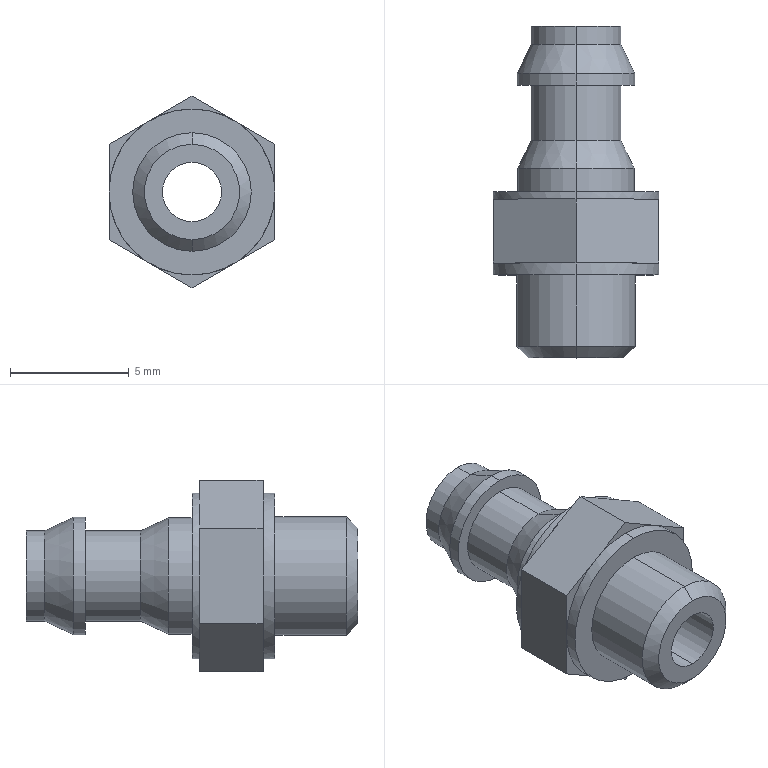Part | STEP file | M-5AU-6 | 1 solid | 45 faces | box 7 x 14 x 8.083 mm | volume 243.361 mm3 | plane 23 | cylinder 16 | cone 6 | commonest cylinder face diameters 3.8 x4 7 x4 2.5 x2 4.9 x2 4.95 x2 5 x2
STEP:
#1=CARTESIAN_POINT('',(0.,14.,1.25));
#2=VERTEX_POINT('',#1);
#3=CARTESIAN_POINT('',(0.,14.,-1.25));
#4=VERTEX_POINT('',#3);
#5=CARTESIAN_POINT('',(0.,14.,0.));
#6=DIRECTION('',(0.,-1.,0.));
#7=DIRECTION('',(0.,0.,-1.));
#8=AXIS2_PLACEMENT_3D('',#5,#6,#7);
#9=CIRCLE('',#8,1.25);
#10=EDGE_CURVE('',#2,#4,#9,.T.);
#11=ORIENTED_EDGE('',*,*,#10,.F.);
#12=CARTESIAN_POINT('',(0.,0.,1.25));
#13=VERTEX_POINT('',#12);
#14=CARTESIAN_POINT('',(0.,0.,1.25));
#15=DIRECTION('',(0.,-1.,0.));
#16=VECTOR('',#15,1000.);
#17=LINE('',#14,#16);
#18=EDGE_CURVE('',#2,#13,#17,.T.);
#19=ORIENTED_EDGE('',*,*,#18,.T.);
#20=CARTESIAN_POINT('',(0.,0.,-1.25));
#21=VERTEX_POINT('',#20);
#22=CARTESIAN_POINT('',(0.,0.,0.));
#23=DIRECTION('',(0.,1.,0.));
#24=DIRECTION('',(0.,0.,-1.));
#25=AXIS2_PLACEMENT_3D('',#22,#23,#24);
#26=CIRCLE('',#25,1.25);
#27=EDGE_CURVE('',#21,#13,#26,.T.);
#28=ORIENTED_EDGE('',*,*,#27,.F.);
#29=CARTESIAN_POINT('',(0.,0.,-1.25));
#30=DIRECTION('',(0.,-1.,0.));
#31=VECTOR('',#30,1000.);
#32=LINE('',#29,#31);
#33=EDGE_CURVE('',#4,#21,#32,.T.);
#34=ORIENTED_EDGE('',*,*,#33,.F.);
#35=EDGE_LOOP('',(#11,#19,#28,#34));
#36=FACE_OUTER_BOUND('',#35,.T.);
#37=CARTESIAN_POINT('',(0.,0.,0.));
#38=DIRECTION('',(0.,-1.,0.));
#39=DIRECTION('',(0.,0.,-1.));
#40=AXIS2_PLACEMENT_3D('',#37,#38,#39);
#41=CYLINDRICAL_SURFACE('',#40,1.25);
#42=ADVANCED_FACE('',(#36),#41,.F.);
#43=CARTESIAN_POINT('',(0.,14.,1.9));
#44=VERTEX_POINT('',#43);
#45=CARTESIAN_POINT('',(0.,14.,-1.9));
#46=VERTEX_POINT('',#45);
#47=CARTESIAN_POINT('',(0.,14.,0.));
#48=DIRECTION('',(0.,1.,0.));
#49=DIRECTION('',(0.,0.,-1.));
#50=AXIS2_PLACEMENT_3D('',#47,#48,#49);
#51=CIRCLE('',#50,1.9);
#52=EDGE_CURVE('',#44,#46,#51,.T.);
#53=ORIENTED_EDGE('',*,*,#52,.F.);
#54=CARTESIAN_POINT('',(0.,13.233,1.9));
#55=VERTEX_POINT('',#54);
#56=CARTESIAN_POINT('',(0.,13.617,1.9));
#57=DIRECTION('',(0.,-1.,0.));
#58=VECTOR('',#57,1000.);
#59=LINE('',#56,#58);
#60=EDGE_CURVE('',#44,#55,#59,.T.);
#61=ORIENTED_EDGE('',*,*,#60,.T.);
#62=CARTESIAN_POINT('',(0.,13.233,-1.9));
#63=VERTEX_POINT('',#62);
#64=CARTESIAN_POINT('',(0.,13.233,0.));
#65=DIRECTION('',(0.,1.,0.));
#66=DIRECTION('',(0.,0.,-1.));
#67=AXIS2_PLACEMENT_3D('',#64,#65,#66);
#68=CIRCLE('',#67,1.9);
#69=EDGE_CURVE('',#55,#63,#68,.T.);
#70=ORIENTED_EDGE('',*,*,#69,.T.);
#71=CARTESIAN_POINT('',(0.,13.617,-1.9));
#72=DIRECTION('',(0.,-1.,0.));
#73=VECTOR('',#72,1000.);
#74=LINE('',#71,#73);
#75=EDGE_CURVE('',#46,#63,#74,.T.);
#76=ORIENTED_EDGE('',*,*,#75,.F.);
#77=EDGE_LOOP('',(#53,#61,#70,#76));
#78=FACE_OUTER_BOUND('',#77,.T.);
#79=CARTESIAN_POINT('',(0.,13.617,0.));
#80=DIRECTION('',(0.,-1.,0.));
#81=DIRECTION('',(0.,0.,-1.));
#82=AXIS2_PLACEMENT_3D('',#79,#80,#81);
#83=CYLINDRICAL_SURFACE('',#82,1.9);
#84=ADVANCED_FACE('',(#78),#83,.T.);
#85=CARTESIAN_POINT('',(0.,0.,-2.01));
#86=VERTEX_POINT('',#85);
#87=CARTESIAN_POINT('',(0.,0.,2.01));
#88=VERTEX_POINT('',#87);
#89=CARTESIAN_POINT('',(0.,0.,0.));
#90=DIRECTION('',(0.,-1.,0.));
#91=DIRECTION('',(0.,0.,1.));
#92=AXIS2_PLACEMENT_3D('',#89,#90,#91);
#93=CIRCLE('',#92,2.01);
#94=EDGE_CURVE('',#86,#88,#93,.T.);
#95=ORIENTED_EDGE('',*,*,#94,.F.);
#96=CARTESIAN_POINT('',(0.,0.49,-2.5));
#97=VERTEX_POINT('',#96);
#98=CARTESIAN_POINT('',(0.,0.49,-2.5));
#99=DIRECTION('',(0.,0.7071,-0.7071));
#100=VECTOR('',#99,1000.);
#101=LINE('',#98,#100);
#102=EDGE_CURVE('',#86,#97,#101,.T.);
#103=ORIENTED_EDGE('',*,*,#102,.T.);
#104=CARTESIAN_POINT('',(0.,0.49,2.5));
#105=VERTEX_POINT('',#104);
#106=CARTESIAN_POINT('',(0.,0.49,0.));
#107=DIRECTION('',(0.,-1.,0.));
#108=DIRECTION('',(1.,0.,0.));
#109=AXIS2_PLACEMENT_3D('',#106,#107,#108);
#110=CIRCLE('',#109,2.5);
#111=EDGE_CURVE('',#97,#105,#110,.T.);
#112=ORIENTED_EDGE('',*,*,#111,.T.);
#113=CARTESIAN_POINT('',(0.,0.49,2.5));
#114=DIRECTION('',(0.,0.7071,0.7071));
#115=VECTOR('',#114,1000.);
#116=LINE('',#113,#115);
#117=EDGE_CURVE('',#88,#105,#116,.T.);
#118=ORIENTED_EDGE('',*,*,#117,.F.);
#119=EDGE_LOOP('',(#95,#103,#112,#118));
#120=FACE_OUTER_BOUND('',#119,.T.);
#121=CARTESIAN_POINT('',(0.,0.49,0.));
#122=DIRECTION('',(0.,1.,0.));
#123=DIRECTION('',(0.,0.,1.));
#124=AXIS2_PLACEMENT_3D('',#121,#122,#123);
#125=CONICAL_SURFACE('',#124,2.5,0.7854);
#126=ADVANCED_FACE('',(#120),#125,.T.);
#127=ORIENTED_EDGE('',*,*,#69,.F.);
#128=CARTESIAN_POINT('',(0.,12.,2.475));
#129=VERTEX_POINT('',#128);
#130=CARTESIAN_POINT('',(0.,12.,2.475));
#131=DIRECTION('',(0.,-0.9063,0.4226));
#132=VECTOR('',#131,1000.);
#133=LINE('',#130,#132);
#134=EDGE_CURVE('',#55,#129,#133,.T.);
#135=ORIENTED_EDGE('',*,*,#134,.T.);
#136=CARTESIAN_POINT('',(0.,12.,-2.475));
#137=VERTEX_POINT('',#136);
#138=CARTESIAN_POINT('',(0.,12.,0.));
#139=DIRECTION('',(0.,1.,0.));
#140=DIRECTION('',(1.,0.,0.));
#141=AXIS2_PLACEMENT_3D('',#138,#139,#140);
#142=CIRCLE('',#141,2.475);
#143=EDGE_CURVE('',#129,#137,#142,.T.);
#144=ORIENTED_EDGE('',*,*,#143,.T.);
#145=CARTESIAN_POINT('',(0.,12.,-2.475));
#146=DIRECTION('',(0.,-0.9063,-0.4226));
#147=VECTOR('',#146,1000.);
#148=LINE('',#145,#147);
#149=EDGE_CURVE('',#63,#137,#148,.T.);
#150=ORIENTED_EDGE('',*,*,#149,.F.);
#151=EDGE_LOOP('',(#127,#135,#144,#150));
#152=FACE_OUTER_BOUND('',#151,.T.);
#153=CARTESIAN_POINT('',(0.,12.,0.));
#154=DIRECTION('',(0.,-1.,0.));
#155=DIRECTION('',(0.,0.,-1.));
#156=AXIS2_PLACEMENT_3D('',#153,#154,#155);
#157=CONICAL_SURFACE('',#156,2.475,0.4363);
#158=ADVANCED_FACE('',(#152),#157,.T.);
#159=CARTESIAN_POINT('',(0.,3.5,-2.5));
#160=VERTEX_POINT('',#159);
#161=CARTESIAN_POINT('',(0.,3.5,2.5));
#162=VERTEX_POINT('',#161);
#163=CARTESIAN_POINT('',(0.,3.5,0.));
#164=DIRECTION('',(0.,-1.,0.));
#165=DIRECTION('',(0.,0.,-1.));
#166=AXIS2_PLACEMENT_3D('',#163,#164,#165);
#167=CIRCLE('',#166,2.5);
#168=EDGE_CURVE('',#160,#162,#167,.T.);
#169=ORIENTED_EDGE('',*,*,#168,.T.);
#170=CARTESIAN_POINT('',(0.,1.995,2.5));
#171=DIRECTION('',(0.,-1.,0.));
#172=VECTOR('',#171,1000.);
#173=LINE('',#170,#172);
#174=EDGE_CURVE('',#162,#105,#173,.T.);
#175=ORIENTED_EDGE('',*,*,#174,.T.);
#176=ORIENTED_EDGE('',*,*,#111,.F.);
#177=CARTESIAN_POINT('',(0.,1.995,-2.5));
#178=DIRECTION('',(0.,-1.,0.));
#179=VECTOR('',#178,1000.);
#180=LINE('',#177,#179);
#181=EDGE_CURVE('',#160,#97,#180,.T.);
#182=ORIENTED_EDGE('',*,*,#181,.F.);
#183=EDGE_LOOP('',(#169,#175,#176,#182));
#184=FACE_OUTER_BOUND('',#183,.T.);
#185=CARTESIAN_POINT('',(0.,1.995,0.));
#186=DIRECTION('',(0.,-1.,0.));
#187=DIRECTION('',(0.,0.,-1.));
#188=AXIS2_PLACEMENT_3D('',#185,#186,#187);
#189=CYLINDRICAL_SURFACE('',#188,2.5);
#190=ADVANCED_FACE('',(#184),#189,.T.);
#191=ORIENTED_EDGE('',*,*,#143,.F.);
#192=CARTESIAN_POINT('',(0.,11.5,2.475));
#193=VERTEX_POINT('',#192);
#194=CARTESIAN_POINT('',(0.,11.75,2.475));
#195=DIRECTION('',(0.,-1.,0.));
#196=VECTOR('',#195,1000.);
#197=LINE('',#194,#196);
#198=EDGE_CURVE('',#129,#193,#197,.T.);
#199=ORIENTED_EDGE('',*,*,#198,.T.);
#200=CARTESIAN_POINT('',(0.,11.5,-2.475));
#201=VERTEX_POINT('',#200);
#202=CARTESIAN_POINT('',(0.,11.5,0.));
#203=DIRECTION('',(0.,1.,0.));
#204=DIRECTION('',(0.,0.,-1.));
#205=AXIS2_PLACEMENT_3D('',#202,#203,#204);
#206=CIRCLE('',#205,2.475);
#207=EDGE_CURVE('',#193,#201,#206,.T.);
#208=ORIENTED_EDGE('',*,*,#207,.T.);
#209=CARTESIAN_POINT('',(0.,11.75,-2.475));
#210=DIRECTION('',(0.,-1.,0.));
#211=VECTOR('',#210,1000.);
#212=LINE('',#209,#211);
#213=EDGE_CURVE('',#137,#201,#212,.T.);
#214=ORIENTED_EDGE('',*,*,#213,.F.);
#215=EDGE_LOOP('',(#191,#199,#208,#214));
#216=FACE_OUTER_BOUND('',#215,.T.);
#217=CARTESIAN_POINT('',(0.,11.75,0.));
#218=DIRECTION('',(0.,-1.,0.));
#219=DIRECTION('',(0.,0.,-1.));
#220=AXIS2_PLACEMENT_3D('',#217,#218,#219);
#221=CYLINDRICAL_SURFACE('',#220,2.475);
#222=ADVANCED_FACE('',(#216),#221,.T.);
#223=CARTESIAN_POINT('',(1.75,4.,3.031));
#224=VERTEX_POINT('',#223);
#225=CARTESIAN_POINT('',(0.,4.,3.5));
#226=VERTEX_POINT('',#225);
#227=CARTESIAN_POINT('',(0.,4.,0.));
#228=DIRECTION('',(0.,-1.,0.));
#229=DIRECTION('',(0.,0.,-1.));
#230=AXIS2_PLACEMENT_3D('',#227,#228,#229);
#231=CIRCLE('',#230,3.5);
#232=EDGE_CURVE('',#224,#226,#231,.T.);
#233=ORIENTED_EDGE('',*,*,#232,.T.);
#234=CARTESIAN_POINT('',(0.,3.5,3.5));
#235=VERTEX_POINT('',#234);
#236=CARTESIAN_POINT('',(0.,3.75,3.5));
#237=DIRECTION('',(0.,-1.,0.));
#238=VECTOR('',#237,1000.);
#239=LINE('',#236,#238);
#240=EDGE_CURVE('',#226,#235,#239,.T.);
#241=ORIENTED_EDGE('',*,*,#240,.T.);
#242=CARTESIAN_POINT('',(0.,3.5,-3.5));
#243=VERTEX_POINT('',#242);
#244=CARTESIAN_POINT('',(0.,3.5,0.));
#245=DIRECTION('',(0.,-1.,0.));
#246=DIRECTION('',(0.,0.,-1.));
#247=AXIS2_PLACEMENT_3D('',#244,#245,#246);
#248=CIRCLE('',#247,3.5);
#249=EDGE_CURVE('',#243,#235,#248,.T.);
#250=ORIENTED_EDGE('',*,*,#249,.F.);
#251=CARTESIAN_POINT('',(0.,4.,-3.5));
#252=VERTEX_POINT('',#251);
#253=CARTESIAN_POINT('',(0.,3.75,-3.5));
#254=DIRECTION('',(0.,-1.,0.));
#255=VECTOR('',#254,1000.);
#256=LINE('',#253,#255);
#257=EDGE_CURVE('',#252,#243,#256,.T.);
#258=ORIENTED_EDGE('',*,*,#257,.F.);
#259=CARTESIAN_POINT('',(1.75,4.,-3.031));
#260=VERTEX_POINT('',#259);
#261=CARTESIAN_POINT('',(0.,4.,0.));
#262=DIRECTION('',(0.,-1.,0.));
#263=DIRECTION('',(0.,0.,-1.));
#264=AXIS2_PLACEMENT_3D('',#261,#262,#263);
#265=CIRCLE('',#264,3.5);
#266=EDGE_CURVE('',#252,#260,#265,.T.);
#267=ORIENTED_EDGE('',*,*,#266,.T.);
#268=CARTESIAN_POINT('',(3.5,4.,0.));
#269=VERTEX_POINT('',#268);
#270=CARTESIAN_POINT('',(0.,4.,0.));
#271=DIRECTION('',(0.,-1.,0.));
#272=DIRECTION('',(0.,0.,-1.));
#273=AXIS2_PLACEMENT_3D('',#270,#271,#272);
#274=CIRCLE('',#273,3.5);
#275=EDGE_CURVE('',#260,#269,#274,.T.);
#276=ORIENTED_EDGE('',*,*,#275,.T.);
#277=CARTESIAN_POINT('',(0.,4.,0.));
#278=DIRECTION('',(0.,-1.,0.));
#279=DIRECTION('',(0.,0.,-1.));
#280=AXIS2_PLACEMENT_3D('',#277,#278,#279);
#281=CIRCLE('',#280,3.5);
#282=EDGE_CURVE('',#269,#224,#281,.T.);
#283=ORIENTED_EDGE('',*,*,#282,.T.);
#284=EDGE_LOOP('',(#233,#241,#250,#258,#267,#276,#283));
#285=FACE_OUTER_BOUND('',#284,.T.);
#286=CARTESIAN_POINT('',(0.,3.75,0.));
#287=DIRECTION('',(0.,-1.,0.));
#288=DIRECTION('',(0.,0.,-1.));
#289=AXIS2_PLACEMENT_3D('',#286,#287,#288);
#290=CYLINDRICAL_SURFACE('',#289,3.5);
#291=ADVANCED_FACE('',(#285),#290,.T.);
#292=CARTESIAN_POINT('',(0.,11.5,1.9));
#293=VERTEX_POINT('',#292);
#294=CARTESIAN_POINT('',(0.,11.5,-1.9));
#295=VERTEX_POINT('',#294);
#296=CARTESIAN_POINT('',(0.,11.5,0.));
#297=DIRECTION('',(0.,1.,0.));
#298=DIRECTION('',(0.,0.,-1.));
#299=AXIS2_PLACEMENT_3D('',#296,#297,#298);
#300=CIRCLE('',#299,1.9);
#301=EDGE_CURVE('',#293,#295,#300,.T.);
#302=ORIENTED_EDGE('',*,*,#301,.F.);
#303=CARTESIAN_POINT('',(0.,9.179,1.9));
#304=VERTEX_POINT('',#303);
#305=CARTESIAN_POINT('',(0.,10.34,1.9));
#306=DIRECTION('',(0.,-1.,0.));
#307=VECTOR('',#306,1000.);
#308=LINE('',#305,#307);
#309=EDGE_CURVE('',#293,#304,#308,.T.);
#310=ORIENTED_EDGE('',*,*,#309,.T.);
#311=CARTESIAN_POINT('',(0.,9.179,-1.9));
#312=VERTEX_POINT('',#311);
#313=CARTESIAN_POINT('',(0.,9.179,0.));
#314=DIRECTION('',(0.,1.,0.));
#315=DIRECTION('',(0.,0.,-1.));
#316=AXIS2_PLACEMENT_3D('',#313,#314,#315);
#317=CIRCLE('',#316,1.9);
#318=EDGE_CURVE('',#304,#312,#317,.T.);
#319=ORIENTED_EDGE('',*,*,#318,.T.);
#320=CARTESIAN_POINT('',(0.,10.34,-1.9));
#321=DIRECTION('',(0.,-1.,0.));
#322=VECTOR('',#321,1000.);
#323=LINE('',#320,#322);
#324=EDGE_CURVE('',#295,#312,#323,.T.);
#325=ORIENTED_EDGE('',*,*,#324,.F.);
#326=EDGE_LOOP('',(#302,#310,#319,#325));
#327=FACE_OUTER_BOUND('',#326,.T.);
#328=CARTESIAN_POINT('',(0.,10.34,0.));
#329=DIRECTION('',(0.,-1.,0.));
#330=DIRECTION('',(0.,0.,-1.));
#331=AXIS2_PLACEMENT_3D('',#328,#329,#330);
#332=CYLINDRICAL_SURFACE('',#331,1.9);
#333=ADVANCED_FACE('',(#327),#332,.T.);
#334=ORIENTED_EDGE('',*,*,#318,.F.);
#335=CARTESIAN_POINT('',(0.,8.,2.45));
#336=VERTEX_POINT('',#335);
#337=CARTESIAN_POINT('',(0.,8.,2.45));
#338=DIRECTION('',(0.,-0.9063,0.4226));
#339=VECTOR('',#338,1000.);
#340=LINE('',#337,#339);
#341=EDGE_CURVE('',#304,#336,#340,.T.);
#342=ORIENTED_EDGE('',*,*,#341,.T.);
#343=CARTESIAN_POINT('',(0.,8.,-2.45));
#344=VERTEX_POINT('',#343);
#345=CARTESIAN_POINT('',(0.,8.,0.));
#346=DIRECTION('',(0.,1.,0.));
#347=DIRECTION('',(1.,0.,0.));
#348=AXIS2_PLACEMENT_3D('',#345,#346,#347);
#349=CIRCLE('',#348,2.45);
#350=EDGE_CURVE('',#336,#344,#349,.T.);
#351=ORIENTED_EDGE('',*,*,#350,.T.);
#352=CARTESIAN_POINT('',(0.,8.,-2.45));
#353=DIRECTION('',(0.,-0.9063,-0.4226));
#354=VECTOR('',#353,1000.);
#355=LINE('',#352,#354);
#356=EDGE_CURVE('',#312,#344,#355,.T.);
#357=ORIENTED_EDGE('',*,*,#356,.F.);
#358=EDGE_LOOP('',(#334,#342,#351,#357));
#359=FACE_OUTER_BOUND('',#358,.T.);
#360=CARTESIAN_POINT('',(0.,8.,0.));
#361=DIRECTION('',(0.,-1.,0.));
#362=DIRECTION('',(0.,0.,-1.));
#363=AXIS2_PLACEMENT_3D('',#360,#361,#362);
#364=CONICAL_SURFACE('',#363,2.45,0.4363);
#365=ADVANCED_FACE('',(#359),#364,.T.);
#366=ORIENTED_EDGE('',*,*,#350,.F.);
#367=CARTESIAN_POINT('',(0.,7.,2.45));
#368=VERTEX_POINT('',#367);
#369=CARTESIAN_POINT('',(0.,7.5,2.45));
#370=DIRECTION('',(0.,-1.,0.));
#371=VECTOR('',#370,1000.);
#372=LINE('',#369,#371);
#373=EDGE_CURVE('',#336,#368,#372,.T.);
#374=ORIENTED_EDGE('',*,*,#373,.T.);
#375=CARTESIAN_POINT('',(0.,7.,-2.45));
#376=VERTEX_POINT('',#375);
#377=CARTESIAN_POINT('',(0.,7.,0.));
#378=DIRECTION('',(0.,1.,0.));
#379=DIRECTION('',(0.,0.,-1.));
#380=AXIS2_PLACEMENT_3D('',#377,#378,#379);
#381=CIRCLE('',#380,2.45);
#382=EDGE_CURVE('',#368,#376,#381,.T.);
#383=ORIENTED_EDGE('',*,*,#382,.T.);
#384=CARTESIAN_POINT('',(0.,7.5,-2.45));
#385=DIRECTION('',(0.,-1.,0.));
#386=VECTOR('',#385,1000.);
#387=LINE('',#384,#386);
#388=EDGE_CURVE('',#344,#376,#387,.T.);
#389=ORIENTED_EDGE('',*,*,#388,.F.);
#390=EDGE_LOOP('',(#366,#374,#383,#389));
#391=FACE_OUTER_BOUND('',#390,.T.);
#392=CARTESIAN_POINT('',(0.,7.5,0.));
#393=DIRECTION('',(0.,-1.,0.));
#394=DIRECTION('',(0.,0.,-1.));
#395=AXIS2_PLACEMENT_3D('',#392,#393,#394);
#396=CYLINDRICAL_SURFACE('',#395,2.45);
#397=ADVANCED_FACE('',(#391),#396,.T.);
#398=CARTESIAN_POINT('',(0.,7.,3.5));
#399=VERTEX_POINT('',#398);
#400=CARTESIAN_POINT('',(0.,7.,-3.5));
#401=VERTEX_POINT('',#400);
#402=CARTESIAN_POINT('',(0.,7.,0.));
#403=DIRECTION('',(0.,1.,0.));
#404=DIRECTION('',(0.,0.,-1.));
#405=AXIS2_PLACEMENT_3D('',#402,#403,#404);
#406=CIRCLE('',#405,3.5);
#407=EDGE_CURVE('',#399,#401,#406,.T.);
#408=ORIENTED_EDGE('',*,*,#407,.F.);
#409=CARTESIAN_POINT('',(0.,6.7,3.5));
#410=VERTEX_POINT('',#409);
#411=CARTESIAN_POINT('',(0.,6.7,3.5));
#412=DIRECTION('',(0.,-1.,0.));
#413=VECTOR('',#412,1000.);
#414=LINE('',#411,#413);
#415=EDGE_CURVE('',#399,#410,#414,.T.);
#416=ORIENTED_EDGE('',*,*,#415,.T.);
#417=CARTESIAN_POINT('',(1.75,6.7,3.031));
#418=VERTEX_POINT('',#417);
#419=CARTESIAN_POINT('',(0.,6.7,0.));
#420=DIRECTION('',(0.,-1.,0.));
#421=DIRECTION('',(0.,0.,-1.));
#422=AXIS2_PLACEMENT_3D('',#419,#420,#421);
#423=CIRCLE('',#422,3.5);
#424=EDGE_CURVE('',#418,#410,#423,.T.);
#425=ORIENTED_EDGE('',*,*,#424,.F.);
#426=CARTESIAN_POINT('',(3.5,6.7,0.));
#427=VERTEX_POINT('',#426);
#428=CARTESIAN_POINT('',(0.,6.7,0.));
#429=DIRECTION('',(0.,-1.,0.));
#430=DIRECTION('',(0.,0.,-1.));
#431=AXIS2_PLACEMENT_3D('',#428,#429,#430);
#432=CIRCLE('',#431,3.5);
#433=EDGE_CURVE('',#427,#418,#432,.T.);
#434=ORIENTED_EDGE('',*,*,#433,.F.);
#435=CARTESIAN_POINT('',(1.75,6.7,-3.031));
#436=VERTEX_POINT('',#435);
#437=CARTESIAN_POINT('',(0.,6.7,0.));
#438=DIRECTION('',(0.,-1.,0.));
#439=DIRECTION('',(0.,0.,-1.));
#440=AXIS2_PLACEMENT_3D('',#437,#438,#439);
#441=CIRCLE('',#440,3.5);
#442=EDGE_CURVE('',#436,#427,#441,.T.);
#443=ORIENTED_EDGE('',*,*,#442,.F.);
#444=CARTESIAN_POINT('',(0.,6.7,-3.5));
#445=VERTEX_POINT('',#444);
#446=CARTESIAN_POINT('',(0.,6.7,0.));
#447=DIRECTION('',(0.,-1.,0.));
#448=DIRECTION('',(0.,0.,-1.));
#449=AXIS2_PLACEMENT_3D('',#446,#447,#448);
#450=CIRCLE('',#449,3.5);
#451=EDGE_CURVE('',#445,#436,#450,.T.);
#452=ORIENTED_EDGE('',*,*,#451,.F.);
#453=CARTESIAN_POINT('',(0.,6.7,-3.5));
#454=DIRECTION('',(0.,-1.,0.));
#455=VECTOR('',#454,1000.);
#456=LINE('',#453,#455);
#457=EDGE_CURVE('',#401,#445,#456,.T.);
#458=ORIENTED_EDGE('',*,*,#457,.F.);
#459=EDGE_LOOP('',(#408,#416,#425,#434,#443,#452,#458));
#460=FACE_OUTER_BOUND('',#459,.T.);
#461=CARTESIAN_POINT('',(0.,6.7,0.));
#462=DIRECTION('',(0.,-1.,0.));
#463=DIRECTION('',(0.,0.,-1.));
#464=AXIS2_PLACEMENT_3D('',#461,#462,#463);
#465=CYLINDRICAL_SURFACE('',#464,3.5);
#466=ADVANCED_FACE('',(#460),#465,.T.);
#467=ORIENTED_EDGE('',*,*,#18,.F.);
#468=CARTESIAN_POINT('',(0.,14.,0.));
#469=DIRECTION('',(0.,-1.,0.));
#470=DIRECTION('',(0.,0.,-1.));
#471=AXIS2_PLACEMENT_3D('',#468,#469,#470);
#472=CIRCLE('',#471,1.25);
#473=EDGE_CURVE('',#4,#2,#472,.T.);
#474=ORIENTED_EDGE('',*,*,#473,.F.);
#475=ORIENTED_EDGE('',*,*,#33,.T.);
#476=CARTESIAN_POINT('',(0.,0.,0.));
#477=DIRECTION('',(0.,1.,0.));
#478=DIRECTION('',(0.,0.,-1.));
#479=AXIS2_PLACEMENT_3D('',#476,#477,#478);
#480=CIRCLE('',#479,1.25);
#481=EDGE_CURVE('',#13,#21,#480,.T.);
#482=ORIENTED_EDGE('',*,*,#481,.F.);
#483=EDGE_LOOP('',(#467,#474,#475,#482));
#484=FACE_OUTER_BOUND('',#483,.T.);
#485=CARTESIAN_POINT('',(0.,0.,0.));
#486=DIRECTION('',(0.,-1.,0.));
#487=DIRECTION('',(0.,0.,-1.));
#488=AXIS2_PLACEMENT_3D('',#485,#486,#487);
#489=CYLINDRICAL_SURFACE('',#488,1.25);
#490=ADVANCED_FACE('',(#484),#489,.F.);
#491=CARTESIAN_POINT('',(0.,14.,0.));
#492=DIRECTION('',(0.,1.,0.));
#493=DIRECTION('',(0.,0.,-1.));
#494=AXIS2_PLACEMENT_3D('',#491,#492,#493);
#495=CIRCLE('',#494,1.9);
#496=EDGE_CURVE('',#46,#44,#495,.T.);
#497=ORIENTED_EDGE('',*,*,#496,.T.);
#498=ORIENTED_EDGE('',*,*,#52,.T.);
#499=EDGE_LOOP('',(#497,#498));
#500=FACE_OUTER_BOUND('',#499,.T.);
#501=ORIENTED_EDGE('',*,*,#473,.T.);
#502=ORIENTED_EDGE('',*,*,#10,.T.);
#503=EDGE_LOOP('',(#501,#502));
#504=FACE_BOUND('',#503,.T.);
#505=CARTESIAN_POINT('',(0.95,14.,0.));
#506=DIRECTION('',(0.,1.,0.));
#507=DIRECTION('',(0.,0.,1.));
#508=AXIS2_PLACEMENT_3D('',#505,#506,#507);
#509=PLANE('',#508);
#510=ADVANCED_FACE('',(#500,#504),#509,.T.);
#511=CARTESIAN_POINT('',(0.,0.,0.));
#512=DIRECTION('',(0.,-1.,0.));
#513=DIRECTION('',(0.,0.,1.));
#514=AXIS2_PLACEMENT_3D('',#511,#512,#513);
#515=CIRCLE('',#514,2.01);
#516=EDGE_CURVE('',#88,#86,#515,.T.);
#517=ORIENTED_EDGE('',*,*,#516,.T.);
#518=ORIENTED_EDGE('',*,*,#94,.T.);
#519=EDGE_LOOP('',(#517,#518));
#520=FACE_OUTER_BOUND('',#519,.T.);
#521=ORIENTED_EDGE('',*,*,#27,.T.);
#522=ORIENTED_EDGE('',*,*,#481,.T.);
#523=EDGE_LOOP('',(#521,#522));
#524=FACE_BOUND('',#523,.T.);
#525=CARTESIAN_POINT('',(1.005,0.,0.));
#526=DIRECTION('',(0.,-1.,0.));
#527=DIRECTION('',(0.,0.,-1.));
#528=AXIS2_PLACEMENT_3D('',#525,#526,#527);
#529=PLANE('',#528);
#530=ADVANCED_FACE('',(#520,#524),#529,.T.);
#531=ORIENTED_EDGE('',*,*,#60,.F.);
#532=ORIENTED_EDGE('',*,*,#496,.F.);
#533=ORIENTED_EDGE('',*,*,#75,.T.);
#534=CARTESIAN_POINT('',(0.,13.233,0.));
#535=DIRECTION('',(0.,1.,0.));
#536=DIRECTION('',(0.,0.,-1.));
#537=AXIS2_PLACEMENT_3D('',#534,#535,#536);
#538=CIRCLE('',#537,1.9);
#539=EDGE_CURVE('',#63,#55,#538,.T.);
#540=ORIENTED_EDGE('',*,*,#539,.T.);
#541=EDGE_LOOP('',(#531,#532,#533,#540));
#542=FACE_OUTER_BOUND('',#541,.T.);
#543=CARTESIAN_POINT('',(0.,13.617,0.));
#544=DIRECTION('',(0.,-1.,0.));
#545=DIRECTION('',(0.,0.,-1.));
#546=AXIS2_PLACEMENT_3D('',#543,#544,#545);
#547=CYLINDRICAL_SURFACE('',#546,1.9);
#548=ADVANCED_FACE('',(#542),#547,.T.);
#549=ORIENTED_EDGE('',*,*,#102,.F.);
#550=ORIENTED_EDGE('',*,*,#516,.F.);
#551=ORIENTED_EDGE('',*,*,#117,.T.);
#552=CARTESIAN_POINT('',(0.,0.49,0.));
#553=DIRECTION('',(0.,-1.,0.));
#554=DIRECTION('',(1.,0.,0.));
#555=AXIS2_PLACEMENT_3D('',#552,#553,#554);
#556=CIRCLE('',#555,2.5);
#557=EDGE_CURVE('',#105,#97,#556,.T.);
#558=ORIENTED_EDGE('',*,*,#557,.T.);
#559=EDGE_LOOP('',(#549,#550,#551,#558));
#560=FACE_OUTER_BOUND('',#559,.T.);
#561=CARTESIAN_POINT('',(0.,0.49,0.));
#562=DIRECTION('',(0.,1.,0.));
#563=DIRECTION('',(0.,0.,1.));
#564=AXIS2_PLACEMENT_3D('',#561,#562,#563);
#565=CONICAL_SURFACE('',#564,2.5,0.7854);
#566=ADVANCED_FACE('',(#560),#565,.T.);
#567=ORIENTED_EDGE('',*,*,#134,.F.);
#568=ORIENTED_EDGE('',*,*,#539,.F.);
#569=ORIENTED_EDGE('',*,*,#149,.T.);
#570=CARTESIAN_POINT('',(0.,12.,0.));
#571=DIRECTION('',(0.,1.,0.));
#572=DIRECTION('',(1.,0.,0.));
#573=AXIS2_PLACEMENT_3D('',#570,#571,#572);
#574=CIRCLE('',#573,2.475);
#575=EDGE_CURVE('',#137,#129,#574,.T.);
#576=ORIENTED_EDGE('',*,*,#575,.T.);
#577=EDGE_LOOP('',(#567,#568,#569,#576));
#578=FACE_OUTER_BOUND('',#577,.T.);
#579=CARTESIAN_POINT('',(0.,12.,0.));
#580=DIRECTION('',(0.,-1.,0.));
#581=DIRECTION('',(0.,0.,-1.));
#582=AXIS2_PLACEMENT_3D('',#579,#580,#581);
#583=CONICAL_SURFACE('',#582,2.475,0.4363);
#584=ADVANCED_FACE('',(#578),#583,.T.);
#585=ORIENTED_EDGE('',*,*,#174,.F.);
#586=CARTESIAN_POINT('',(0.,3.5,0.));
#587=DIRECTION('',(0.,-1.,0.));
#588=DIRECTION('',(0.,0.,-1.));
#589=AXIS2_PLACEMENT_3D('',#586,#587,#588);
#590=CIRCLE('',#589,2.5);
#591=EDGE_CURVE('',#162,#160,#590,.T.);
#592=ORIENTED_EDGE('',*,*,#591,.T.);
#593=ORIENTED_EDGE('',*,*,#181,.T.);
#594=ORIENTED_EDGE('',*,*,#557,.F.);
#595=EDGE_LOOP('',(#585,#592,#593,#594));
#596=FACE_OUTER_BOUND('',#595,.T.);
#597=CARTESIAN_POINT('',(0.,1.995,0.));
#598=DIRECTION('',(0.,-1.,0.));
#599=DIRECTION('',(0.,0.,-1.));
#600=AXIS2_PLACEMENT_3D('',#597,#598,#599);
#601=CYLINDRICAL_SURFACE('',#600,2.5);
#602=ADVANCED_FACE('',(#596),#601,.T.);
#603=ORIENTED_EDGE('',*,*,#198,.F.);
#604=ORIENTED_EDGE('',*,*,#575,.F.);
#605=ORIENTED_EDGE('',*,*,#213,.T.);
#606=CARTESIAN_POINT('',(0.,11.5,0.));
#607=DIRECTION('',(0.,1.,0.));
#608=DIRECTION('',(0.,0.,-1.));
#609=AXIS2_PLACEMENT_3D('',#606,#607,#608);
#610=CIRCLE('',#609,2.475);
#611=EDGE_CURVE('',#201,#193,#610,.T.);
#612=ORIENTED_EDGE('',*,*,#611,.T.);
#613=EDGE_LOOP('',(#603,#604,#605,#612));
#614=FACE_OUTER_BOUND('',#613,.T.);
#615=CARTESIAN_POINT('',(0.,11.75,0.));
#616=DIRECTION('',(0.,-1.,0.));
#617=DIRECTION('',(0.,0.,-1.));
#618=AXIS2_PLACEMENT_3D('',#615,#616,#617);
#619=CYLINDRICAL_SURFACE('',#618,2.475);
#620=ADVANCED_FACE('',(#614),#619,.T.);
#621=ORIENTED_EDGE('',*,*,#168,.F.);
#622=ORIENTED_EDGE('',*,*,#591,.F.);
#623=EDGE_LOOP('',(#621,#622));
#624=FACE_BOUND('',#623,.T.);
#625=ORIENTED_EDGE('',*,*,#249,.T.);
#626=CARTESIAN_POINT('',(0.,3.5,0.));
#627=DIRECTION('',(0.,-1.,0.));
#628=DIRECTION('',(0.,0.,-1.));
#629=AXIS2_PLACEMENT_3D('',#626,#627,#628);
#630=CIRCLE('',#629,3.5);
#631=EDGE_CURVE('',#235,#243,#630,.T.);
#632=ORIENTED_EDGE('',*,*,#631,.T.);
#633=EDGE_LOOP('',(#625,#632));
#634=FACE_OUTER_BOUND('',#633,.T.);
#635=CARTESIAN_POINT('',(3.,3.5,0.));
#636=DIRECTION('',(0.,-1.,0.));
#637=DIRECTION('',(0.,0.,-1.));
#638=AXIS2_PLACEMENT_3D('',#635,#636,#637);
#639=PLANE('',#638);
#640=ADVANCED_FACE('',(#624,#634),#639,.T.);
#641=CARTESIAN_POINT('',(0.,11.5,0.));
#642=DIRECTION('',(0.,1.,0.));
#643=DIRECTION('',(0.,0.,-1.));
#644=AXIS2_PLACEMENT_3D('',#641,#642,#643);
#645=CIRCLE('',#644,1.9);
#646=EDGE_CURVE('',#295,#293,#645,.T.);
#647=ORIENTED_EDGE('',*,*,#646,.T.);
#648=ORIENTED_EDGE('',*,*,#301,.T.);
#649=EDGE_LOOP('',(#647,#648));
#650=FACE_BOUND('',#649,.T.);
#651=ORIENTED_EDGE('',*,*,#611,.F.);
#652=ORIENTED_EDGE('',*,*,#207,.F.);
#653=EDGE_LOOP('',(#651,#652));
#654=FACE_OUTER_BOUND('',#653,.T.);
#655=CARTESIAN_POINT('',(2.188,11.5,0.));
#656=DIRECTION('',(0.,-1.,0.));
#657=DIRECTION('',(0.,0.,-1.));
#658=AXIS2_PLACEMENT_3D('',#655,#656,#657);
#659=PLANE('',#658);
#660=ADVANCED_FACE('',(#650,#654),#659,.T.);
#661=ORIENTED_EDGE('',*,*,#240,.F.);
#662=CARTESIAN_POINT('',(-1.75,4.,3.031));
#663=VERTEX_POINT('',#662);
#664=CARTESIAN_POINT('',(0.,4.,0.));
#665=DIRECTION('',(0.,-1.,0.));
#666=DIRECTION('',(0.,0.,-1.));
#667=AXIS2_PLACEMENT_3D('',#664,#665,#666);
#668=CIRCLE('',#667,3.5);
#669=EDGE_CURVE('',#226,#663,#668,.T.);
#670=ORIENTED_EDGE('',*,*,#669,.T.);
#671=CARTESIAN_POINT('',(-3.5,4.,0.));
#672=VERTEX_POINT('',#671);
#673=CARTESIAN_POINT('',(0.,4.,0.));
#674=DIRECTION('',(0.,-1.,0.));
#675=DIRECTION('',(0.,0.,-1.));
#676=AXIS2_PLACEMENT_3D('',#673,#674,#675);
#677=CIRCLE('',#676,3.5);
#678=EDGE_CURVE('',#663,#672,#677,.T.);
#679=ORIENTED_EDGE('',*,*,#678,.T.);
#680=CARTESIAN_POINT('',(-1.75,4.,-3.031));
#681=VERTEX_POINT('',#680);
#682=CARTESIAN_POINT('',(0.,4.,0.));
#683=DIRECTION('',(0.,-1.,0.));
#684=DIRECTION('',(0.,0.,-1.));
#685=AXIS2_PLACEMENT_3D('',#682,#683,#684);
#686=CIRCLE('',#685,3.5);
#687=EDGE_CURVE('',#672,#681,#686,.T.);
#688=ORIENTED_EDGE('',*,*,#687,.T.);
#689=CARTESIAN_POINT('',(0.,4.,0.));
#690=DIRECTION('',(0.,-1.,0.));
#691=DIRECTION('',(0.,0.,-1.));
#692=AXIS2_PLACEMENT_3D('',#689,#690,#691);
#693=CIRCLE('',#692,3.5);
#694=EDGE_CURVE('',#681,#252,#693,.T.);
#695=ORIENTED_EDGE('',*,*,#694,.T.);
#696=ORIENTED_EDGE('',*,*,#257,.T.);
#697=ORIENTED_EDGE('',*,*,#631,.F.);
#698=EDGE_LOOP('',(#661,#670,#679,#688,#695,#696,#697));
#699=FACE_OUTER_BOUND('',#698,.T.);
#700=CARTESIAN_POINT('',(0.,3.75,0.));
#701=DIRECTION('',(0.,-1.,0.));
#702=DIRECTION('',(0.,0.,-1.));
#703=AXIS2_PLACEMENT_3D('',#700,#701,#702);
#704=CYLINDRICAL_SURFACE('',#703,3.5);
#705=ADVANCED_FACE('',(#699),#704,.T.);
#706=ORIENTED_EDGE('',*,*,#309,.F.);
#707=ORIENTED_EDGE('',*,*,#646,.F.);
#708=ORIENTED_EDGE('',*,*,#324,.T.);
#709=CARTESIAN_POINT('',(0.,9.179,0.));
#710=DIRECTION('',(0.,1.,0.));
#711=DIRECTION('',(0.,0.,-1.));
#712=AXIS2_PLACEMENT_3D('',#709,#710,#711);
#713=CIRCLE('',#712,1.9);
#714=EDGE_CURVE('',#312,#304,#713,.T.);
#715=ORIENTED_EDGE('',*,*,#714,.T.);
#716=EDGE_LOOP('',(#706,#707,#708,#715));
#717=FACE_OUTER_BOUND('',#716,.T.);
#718=CARTESIAN_POINT('',(0.,10.34,0.));
#719=DIRECTION('',(0.,-1.,0.));
#720=DIRECTION('',(0.,0.,-1.));
#721=AXIS2_PLACEMENT_3D('',#718,#719,#720);
#722=CYLINDRICAL_SURFACE('',#721,1.9);
#723=ADVANCED_FACE('',(#717),#722,.T.);
#724=CARTESIAN_POINT('',(-3.5,4.,2.021));
#725=VERTEX_POINT('',#724);
#726=CARTESIAN_POINT('',(-3.5,4.,2.021));
#727=DIRECTION('',(0.866,0.,0.5));
#728=VECTOR('',#727,1000.);
#729=LINE('',#726,#728);
#730=EDGE_CURVE('',#725,#663,#729,.T.);
#731=ORIENTED_EDGE('',*,*,#730,.F.);
#732=CARTESIAN_POINT('',(-3.5,4.,0.));
#733=DIRECTION('',(0.,0.,1.));
#734=VECTOR('',#733,1000.);
#735=LINE('',#732,#734);
#736=EDGE_CURVE('',#672,#725,#735,.T.);
#737=ORIENTED_EDGE('',*,*,#736,.F.);
#738=ORIENTED_EDGE('',*,*,#678,.F.);
#739=EDGE_LOOP('',(#731,#737,#738));
#740=FACE_OUTER_BOUND('',#739,.T.);
#741=CARTESIAN_POINT('',(0.,4.,0.));
#742=DIRECTION('',(0.,1.,0.));
#743=DIRECTION('',(0.,0.,1.));
#744=AXIS2_PLACEMENT_3D('',#741,#742,#743);
#745=PLANE('',#744);
#746=ADVANCED_FACE('',(#740),#745,.F.);
#747=CARTESIAN_POINT('',(0.,4.,4.041));
#748=VERTEX_POINT('',#747);
#749=CARTESIAN_POINT('',(0.,4.,4.041));
#750=DIRECTION('',(0.866,0.,-0.5));
#751=VECTOR('',#750,1000.);
#752=LINE('',#749,#751);
#753=EDGE_CURVE('',#748,#224,#752,.T.);
#754=ORIENTED_EDGE('',*,*,#753,.F.);
#755=CARTESIAN_POINT('',(-1.75,4.,3.031));
#756=DIRECTION('',(0.866,0.,0.5));
#757=VECTOR('',#756,1000.);
#758=LINE('',#755,#757);
#759=EDGE_CURVE('',#663,#748,#758,.T.);
#760=ORIENTED_EDGE('',*,*,#759,.F.);
#761=ORIENTED_EDGE('',*,*,#669,.F.);
#762=ORIENTED_EDGE('',*,*,#232,.F.);
#763=EDGE_LOOP('',(#754,#760,#761,#762));
#764=FACE_OUTER_BOUND('',#763,.T.);
#765=CARTESIAN_POINT('',(0.,4.,0.));
#766=DIRECTION('',(0.,1.,0.));
#767=DIRECTION('',(0.,0.,1.));
#768=AXIS2_PLACEMENT_3D('',#765,#766,#767);
#769=PLANE('',#768);
#770=ADVANCED_FACE('',(#764),#769,.F.);
#771=CARTESIAN_POINT('',(3.5,4.,2.021));
#772=VERTEX_POINT('',#771);
#773=CARTESIAN_POINT('',(3.5,4.,0.));
#774=DIRECTION('',(0.,0.,-1.));
#775=VECTOR('',#774,1000.);
#776=LINE('',#773,#775);
#777=EDGE_CURVE('',#772,#269,#776,.T.);
#778=ORIENTED_EDGE('',*,*,#777,.F.);
#779=CARTESIAN_POINT('',(1.75,4.,3.031));
#780=DIRECTION('',(0.866,0.,-0.5));
#781=VECTOR('',#780,1000.);
#782=LINE('',#779,#781);
#783=EDGE_CURVE('',#224,#772,#782,.T.);
#784=ORIENTED_EDGE('',*,*,#783,.F.);
#785=ORIENTED_EDGE('',*,*,#282,.F.);
#786=EDGE_LOOP('',(#778,#784,#785));
#787=FACE_OUTER_BOUND('',#786,.T.);
#788=CARTESIAN_POINT('',(0.,4.,0.));
#789=DIRECTION('',(0.,1.,0.));
#790=DIRECTION('',(0.,0.,1.));
#791=AXIS2_PLACEMENT_3D('',#788,#789,#790);
#792=PLANE('',#791);
#793=ADVANCED_FACE('',(#787),#792,.F.);
#794=CARTESIAN_POINT('',(3.5,4.,-2.021));
#795=VERTEX_POINT('',#794);
#796=CARTESIAN_POINT('',(3.5,4.,-2.021));
#797=DIRECTION('',(-0.866,0.,-0.5));
#798=VECTOR('',#797,1000.);
#799=LINE('',#796,#798);
#800=EDGE_CURVE('',#795,#260,#799,.T.);
#801=ORIENTED_EDGE('',*,*,#800,.F.);
#802=CARTESIAN_POINT('',(3.5,4.,0.));
#803=DIRECTION('',(0.,0.,-1.));
#804=VECTOR('',#803,1000.);
#805=LINE('',#802,#804);
#806=EDGE_CURVE('',#269,#795,#805,.T.);
#807=ORIENTED_EDGE('',*,*,#806,.F.);
#808=ORIENTED_EDGE('',*,*,#275,.F.);
#809=EDGE_LOOP('',(#801,#807,#808));
#810=FACE_OUTER_BOUND('',#809,.T.);
#811=CARTESIAN_POINT('',(0.,4.,0.));
#812=DIRECTION('',(0.,1.,0.));
#813=DIRECTION('',(0.,0.,1.));
#814=AXIS2_PLACEMENT_3D('',#811,#812,#813);
#815=PLANE('',#814);
#816=ADVANCED_FACE('',(#810),#815,.F.);
#817=CARTESIAN_POINT('',(0.,4.,-4.041));
#818=VERTEX_POINT('',#817);
#819=CARTESIAN_POINT('',(0.,4.,-4.041));
#820=DIRECTION('',(-0.866,0.,0.5));
#821=VECTOR('',#820,1000.);
#822=LINE('',#819,#821);
#823=EDGE_CURVE('',#818,#681,#822,.T.);
#824=ORIENTED_EDGE('',*,*,#823,.F.);
#825=CARTESIAN_POINT('',(1.75,4.,-3.031));
#826=DIRECTION('',(-0.866,0.,-0.5));
#827=VECTOR('',#826,1000.);
#828=LINE('',#825,#827);
#829=EDGE_CURVE('',#260,#818,#828,.T.);
#830=ORIENTED_EDGE('',*,*,#829,.F.);
#831=ORIENTED_EDGE('',*,*,#266,.F.);
#832=ORIENTED_EDGE('',*,*,#694,.F.);
#833=EDGE_LOOP('',(#824,#830,#831,#832));
#834=FACE_OUTER_BOUND('',#833,.T.);
#835=CARTESIAN_POINT('',(0.,4.,0.));
#836=DIRECTION('',(0.,1.,0.));
#837=DIRECTION('',(0.,0.,1.));
#838=AXIS2_PLACEMENT_3D('',#835,#836,#837);
#839=PLANE('',#838);
#840=ADVANCED_FACE('',(#834),#839,.F.);
#841=CARTESIAN_POINT('',(-3.5,4.,-2.021));
#842=VERTEX_POINT('',#841);
#843=CARTESIAN_POINT('',(-3.5,4.,0.));
#844=DIRECTION('',(0.,0.,1.));
#845=VECTOR('',#844,1000.);
#846=LINE('',#843,#845);
#847=EDGE_CURVE('',#842,#672,#846,.T.);
#848=ORIENTED_EDGE('',*,*,#847,.F.);
#849=CARTESIAN_POINT('',(-1.75,4.,-3.031));
#850=DIRECTION('',(-0.866,0.,0.5));
#851=VECTOR('',#850,1000.);
#852=LINE('',#849,#851);
#853=EDGE_CURVE('',#681,#842,#852,.T.);
#854=ORIENTED_EDGE('',*,*,#853,.F.);
#855=ORIENTED_EDGE('',*,*,#687,.F.);
#856=EDGE_LOOP('',(#848,#854,#855));
#857=FACE_OUTER_BOUND('',#856,.T.);
#858=CARTESIAN_POINT('',(0.,4.,0.));
#859=DIRECTION('',(0.,1.,0.));
#860=DIRECTION('',(0.,0.,1.));
#861=AXIS2_PLACEMENT_3D('',#858,#859,#860);
#862=PLANE('',#861);
#863=ADVANCED_FACE('',(#857),#862,.F.);
#864=ORIENTED_EDGE('',*,*,#341,.F.);
#865=ORIENTED_EDGE('',*,*,#714,.F.);
#866=ORIENTED_EDGE('',*,*,#356,.T.);
#867=CARTESIAN_POINT('',(0.,8.,0.));
#868=DIRECTION('',(0.,1.,0.));
#869=DIRECTION('',(1.,0.,0.));
#870=AXIS2_PLACEMENT_3D('',#867,#868,#869);
#871=CIRCLE('',#870,2.45);
#872=EDGE_CURVE('',#344,#336,#871,.T.);
#873=ORIENTED_EDGE('',*,*,#872,.T.);
#874=EDGE_LOOP('',(#864,#865,#866,#873));
#875=FACE_OUTER_BOUND('',#874,.T.);
#876=CARTESIAN_POINT('',(0.,8.,0.));
#877=DIRECTION('',(0.,-1.,0.));
#878=DIRECTION('',(0.,0.,-1.));
#879=AXIS2_PLACEMENT_3D('',#876,#877,#878);
#880=CONICAL_SURFACE('',#879,2.45,0.4363);
#881=ADVANCED_FACE('',(#875),#880,.T.);
#882=ORIENTED_EDGE('',*,*,#759,.T.);
#883=CARTESIAN_POINT('',(0.,6.7,4.041));
#884=VERTEX_POINT('',#883);
#885=CARTESIAN_POINT('',(0.,4.,4.041));
#886=DIRECTION('',(0.,1.,0.));
#887=VECTOR('',#886,1000.);
#888=LINE('',#885,#887);
#889=EDGE_CURVE('',#748,#884,#888,.T.);
#890=ORIENTED_EDGE('',*,*,#889,.T.);
#891=CARTESIAN_POINT('',(-1.75,6.7,3.031));
#892=VERTEX_POINT('',#891);
#893=CARTESIAN_POINT('',(0.,6.7,4.041));
#894=DIRECTION('',(-0.866,0.,-0.5));
#895=VECTOR('',#894,1000.);
#896=LINE('',#893,#895);
#897=EDGE_CURVE('',#884,#892,#896,.T.);
#898=ORIENTED_EDGE('',*,*,#897,.T.);
#899=CARTESIAN_POINT('',(-3.5,6.7,2.021));
#900=VERTEX_POINT('',#899);
#901=CARTESIAN_POINT('',(0.,6.7,4.041));
#902=DIRECTION('',(-0.866,0.,-0.5));
#903=VECTOR('',#902,1000.);
#904=LINE('',#901,#903);
#905=EDGE_CURVE('',#892,#900,#904,.T.);
#906=ORIENTED_EDGE('',*,*,#905,.T.);
#907=CARTESIAN_POINT('',(-3.5,4.,2.021));
#908=DIRECTION('',(0.,-1.,0.));
#909=VECTOR('',#908,1000.);
#910=LINE('',#907,#909);
#911=EDGE_CURVE('',#900,#725,#910,.T.);
#912=ORIENTED_EDGE('',*,*,#911,.T.);
#913=ORIENTED_EDGE('',*,*,#730,.T.);
#914=EDGE_LOOP('',(#882,#890,#898,#906,#912,#913));
#915=FACE_OUTER_BOUND('',#914,.T.);
#916=CARTESIAN_POINT('',(0.,4.,4.041));
#917=DIRECTION('',(-0.5,0.,0.866));
#918=DIRECTION('',(0.866,0.,0.5));
#919=AXIS2_PLACEMENT_3D('',#916,#917,#918);
#920=PLANE('',#919);
#921=ADVANCED_FACE('',(#915),#920,.T.);
#922=ORIENTED_EDGE('',*,*,#736,.T.);
#923=ORIENTED_EDGE('',*,*,#911,.F.);
#924=CARTESIAN_POINT('',(-3.5,6.7,0.));
#925=VERTEX_POINT('',#924);
#926=CARTESIAN_POINT('',(-3.5,6.7,2.021));
#927=DIRECTION('',(0.,0.,-1.));
#928=VECTOR('',#927,1000.);
#929=LINE('',#926,#928);
#930=EDGE_CURVE('',#900,#925,#929,.T.);
#931=ORIENTED_EDGE('',*,*,#930,.T.);
#932=CARTESIAN_POINT('',(-3.5,6.7,-2.021));
#933=VERTEX_POINT('',#932);
#934=CARTESIAN_POINT('',(-3.5,6.7,2.021));
#935=DIRECTION('',(0.,0.,-1.));
#936=VECTOR('',#935,1000.);
#937=LINE('',#934,#936);
#938=EDGE_CURVE('',#925,#933,#937,.T.);
#939=ORIENTED_EDGE('',*,*,#938,.T.);
#940=CARTESIAN_POINT('',(-3.5,4.,-2.021));
#941=DIRECTION('',(0.,-1.,0.));
#942=VECTOR('',#941,1000.);
#943=LINE('',#940,#942);
#944=EDGE_CURVE('',#933,#842,#943,.T.);
#945=ORIENTED_EDGE('',*,*,#944,.T.);
#946=ORIENTED_EDGE('',*,*,#847,.T.);
#947=EDGE_LOOP('',(#922,#923,#931,#939,#945,#946));
#948=FACE_OUTER_BOUND('',#947,.T.);
#949=CARTESIAN_POINT('',(-3.5,4.,2.021));
#950=DIRECTION('',(-1.,0.,0.));
#951=DIRECTION('',(0.,0.,1.));
#952=AXIS2_PLACEMENT_3D('',#949,#950,#951);
#953=PLANE('',#952);
#954=ADVANCED_FACE('',(#948),#953,.T.);
#955=ORIENTED_EDGE('',*,*,#783,.T.);
#956=CARTESIAN_POINT('',(3.5,6.7,2.021));
#957=VERTEX_POINT('',#956);
#958=CARTESIAN_POINT('',(3.5,4.,2.021));
#959=DIRECTION('',(0.,1.,0.));
#960=VECTOR('',#959,1000.);
#961=LINE('',#958,#960);
#962=EDGE_CURVE('',#772,#957,#961,.T.);
#963=ORIENTED_EDGE('',*,*,#962,.T.);
#964=CARTESIAN_POINT('',(3.5,6.7,2.021));
#965=DIRECTION('',(-0.866,0.,0.5));
#966=VECTOR('',#965,1000.);
#967=LINE('',#964,#966);
#968=EDGE_CURVE('',#957,#418,#967,.T.);
#969=ORIENTED_EDGE('',*,*,#968,.T.);
#970=CARTESIAN_POINT('',(3.5,6.7,2.021));
#971=DIRECTION('',(-0.866,0.,0.5));
#972=VECTOR('',#971,1000.);
#973=LINE('',#970,#972);
#974=EDGE_CURVE('',#418,#884,#973,.T.);
#975=ORIENTED_EDGE('',*,*,#974,.T.);
#976=ORIENTED_EDGE('',*,*,#889,.F.);
#977=ORIENTED_EDGE('',*,*,#753,.T.);
#978=EDGE_LOOP('',(#955,#963,#969,#975,#976,#977));
#979=FACE_OUTER_BOUND('',#978,.T.);
#980=CARTESIAN_POINT('',(3.5,4.,2.021));
#981=DIRECTION('',(0.5,0.,0.866));
#982=DIRECTION('',(0.866,0.,-0.5));
#983=AXIS2_PLACEMENT_3D('',#980,#981,#982);
#984=PLANE('',#983);
#985=ADVANCED_FACE('',(#979),#984,.T.);
#986=ORIENTED_EDGE('',*,*,#806,.T.);
#987=CARTESIAN_POINT('',(3.5,6.7,-2.021));
#988=VERTEX_POINT('',#987);
#989=CARTESIAN_POINT('',(3.5,4.,-2.021));
#990=DIRECTION('',(0.,1.,0.));
#991=VECTOR('',#990,1000.);
#992=LINE('',#989,#991);
#993=EDGE_CURVE('',#795,#988,#992,.T.);
#994=ORIENTED_EDGE('',*,*,#993,.T.);
#995=CARTESIAN_POINT('',(3.5,6.7,-2.021));
#996=DIRECTION('',(0.,0.,1.));
#997=VECTOR('',#996,1000.);
#998=LINE('',#995,#997);
#999=EDGE_CURVE('',#988,#427,#998,.T.);
#1000=ORIENTED_EDGE('',*,*,#999,.T.);
#1001=CARTESIAN_POINT('',(3.5,6.7,-2.021));
#1002=DIRECTION('',(0.,0.,1.));
#1003=VECTOR('',#1002,1000.);
#1004=LINE('',#1001,#1003);
#1005=EDGE_CURVE('',#427,#957,#1004,.T.);
#1006=ORIENTED_EDGE('',*,*,#1005,.T.);
#1007=ORIENTED_EDGE('',*,*,#962,.F.);
#1008=ORIENTED_EDGE('',*,*,#777,.T.);
#1009=EDGE_LOOP('',(#986,#994,#1000,#1006,#1007,#1008));
#1010=FACE_OUTER_BOUND('',#1009,.T.);
#1011=CARTESIAN_POINT('',(3.5,4.,-2.021));
#1012=DIRECTION('',(1.,0.,0.));
#1013=DIRECTION('',(0.,0.,-1.));
#1014=AXIS2_PLACEMENT_3D('',#1011,#1012,#1013);
#1015=PLANE('',#1014);
#1016=ADVANCED_FACE('',(#1010),#1015,.T.);
#1017=ORIENTED_EDGE('',*,*,#829,.T.);
#1018=CARTESIAN_POINT('',(0.,6.7,-4.041));
#1019=VERTEX_POINT('',#1018);
#1020=CARTESIAN_POINT('',(0.,4.,-4.041));
#1021=DIRECTION('',(0.,1.,0.));
#1022=VECTOR('',#1021,1000.);
#1023=LINE('',#1020,#1022);
#1024=EDGE_CURVE('',#818,#1019,#1023,.T.);
#1025=ORIENTED_EDGE('',*,*,#1024,.T.);
#1026=CARTESIAN_POINT('',(0.,6.7,-4.041));
#1027=DIRECTION('',(0.866,0.,0.5));
#1028=VECTOR('',#1027,1000.);
#1029=LINE('',#1026,#1028);
#1030=EDGE_CURVE('',#1019,#436,#1029,.T.);
#1031=ORIENTED_EDGE('',*,*,#1030,.T.);
#1032=CARTESIAN_POINT('',(0.,6.7,-4.041));
#1033=DIRECTION('',(0.866,0.,0.5));
#1034=VECTOR('',#1033,1000.);
#1035=LINE('',#1032,#1034);
#1036=EDGE_CURVE('',#436,#988,#1035,.T.);
#1037=ORIENTED_EDGE('',*,*,#1036,.T.);
#1038=ORIENTED_EDGE('',*,*,#993,.F.);
#1039=ORIENTED_EDGE('',*,*,#800,.T.);
#1040=EDGE_LOOP('',(#1017,#1025,#1031,#1037,#1038,#1039));
#1041=FACE_OUTER_BOUND('',#1040,.T.);
#1042=CARTESIAN_POINT('',(0.,4.,-4.041));
#1043=DIRECTION('',(0.5,0.,-0.866));
#1044=DIRECTION('',(-0.866,0.,-0.5));
#1045=AXIS2_PLACEMENT_3D('',#1042,#1043,#1044);
#1046=PLANE('',#1045);
#1047=ADVANCED_FACE('',(#1041),#1046,.T.);
#1048=ORIENTED_EDGE('',*,*,#853,.T.);
#1049=ORIENTED_EDGE('',*,*,#944,.F.);
#1050=CARTESIAN_POINT('',(-1.75,6.7,-3.031));
#1051=VERTEX_POINT('',#1050);
#1052=CARTESIAN_POINT('',(-3.5,6.7,-2.021));
#1053=DIRECTION('',(0.866,0.,-0.5));
#1054=VECTOR('',#1053,1000.);
#1055=LINE('',#1052,#1054);
#1056=EDGE_CURVE('',#933,#1051,#1055,.T.);
#1057=ORIENTED_EDGE('',*,*,#1056,.T.);
#1058=CARTESIAN_POINT('',(-3.5,6.7,-2.021));
#1059=DIRECTION('',(0.866,0.,-0.5));
#1060=VECTOR('',#1059,1000.);
#1061=LINE('',#1058,#1060);
#1062=EDGE_CURVE('',#1051,#1019,#1061,.T.);
#1063=ORIENTED_EDGE('',*,*,#1062,.T.);
#1064=ORIENTED_EDGE('',*,*,#1024,.F.);
#1065=ORIENTED_EDGE('',*,*,#823,.T.);
#1066=EDGE_LOOP('',(#1048,#1049,#1057,#1063,#1064,#1065));
#1067=FACE_OUTER_BOUND('',#1066,.T.);
#1068=CARTESIAN_POINT('',(-3.5,4.,-2.021));
#1069=DIRECTION('',(-0.5,0.,-0.866));
#1070=DIRECTION('',(-0.866,0.,0.5));
#1071=AXIS2_PLACEMENT_3D('',#1068,#1069,#1070);
#1072=PLANE('',#1071);
#1073=ADVANCED_FACE('',(#1067),#1072,.T.);
#1074=ORIENTED_EDGE('',*,*,#373,.F.);
#1075=ORIENTED_EDGE('',*,*,#872,.F.);
#1076=ORIENTED_EDGE('',*,*,#388,.T.);
#1077=CARTESIAN_POINT('',(0.,7.,0.));
#1078=DIRECTION('',(0.,1.,0.));
#1079=DIRECTION('',(0.,0.,-1.));
#1080=AXIS2_PLACEMENT_3D('',#1077,#1078,#1079);
#1081=CIRCLE('',#1080,2.45);
#1082=EDGE_CURVE('',#376,#368,#1081,.T.);
#1083=ORIENTED_EDGE('',*,*,#1082,.T.);
#1084=EDGE_LOOP('',(#1074,#1075,#1076,#1083));
#1085=FACE_OUTER_BOUND('',#1084,.T.);
#1086=CARTESIAN_POINT('',(0.,7.5,0.));
#1087=DIRECTION('',(0.,-1.,0.));
#1088=DIRECTION('',(0.,0.,-1.));
#1089=AXIS2_PLACEMENT_3D('',#1086,#1087,#1088);
#1090=CYLINDRICAL_SURFACE('',#1089,2.45);
#1091=ADVANCED_FACE('',(#1085),#1090,.T.);
#1092=ORIENTED_EDGE('',*,*,#930,.F.);
#1093=ORIENTED_EDGE('',*,*,#905,.F.);
#1094=CARTESIAN_POINT('',(0.,6.7,0.));
#1095=DIRECTION('',(0.,-1.,0.));
#1096=DIRECTION('',(0.,0.,-1.));
#1097=AXIS2_PLACEMENT_3D('',#1094,#1095,#1096);
#1098=CIRCLE('',#1097,3.5);
#1099=EDGE_CURVE('',#892,#925,#1098,.T.);
#1100=ORIENTED_EDGE('',*,*,#1099,.T.);
#1101=EDGE_LOOP('',(#1092,#1093,#1100));
#1102=FACE_OUTER_BOUND('',#1101,.T.);
#1103=CARTESIAN_POINT('',(0.,6.7,0.));
#1104=DIRECTION('',(0.,1.,0.));
#1105=DIRECTION('',(0.,0.,1.));
#1106=AXIS2_PLACEMENT_3D('',#1103,#1104,#1105);
#1107=PLANE('',#1106);
#1108=ADVANCED_FACE('',(#1102),#1107,.T.);
#1109=ORIENTED_EDGE('',*,*,#897,.F.);
#1110=ORIENTED_EDGE('',*,*,#974,.F.);
#1111=ORIENTED_EDGE('',*,*,#424,.T.);
#1112=CARTESIAN_POINT('',(0.,6.7,0.));
#1113=DIRECTION('',(0.,-1.,0.));
#1114=DIRECTION('',(0.,0.,-1.));
#1115=AXIS2_PLACEMENT_3D('',#1112,#1113,#1114);
#1116=CIRCLE('',#1115,3.5);
#1117=EDGE_CURVE('',#410,#892,#1116,.T.);
#1118=ORIENTED_EDGE('',*,*,#1117,.T.);
#1119=EDGE_LOOP('',(#1109,#1110,#1111,#1118));
#1120=FACE_OUTER_BOUND('',#1119,.T.);
#1121=CARTESIAN_POINT('',(0.,6.7,0.));
#1122=DIRECTION('',(0.,1.,0.));
#1123=DIRECTION('',(0.,0.,1.));
#1124=AXIS2_PLACEMENT_3D('',#1121,#1122,#1123);
#1125=PLANE('',#1124);
#1126=ADVANCED_FACE('',(#1120),#1125,.T.);
#1127=ORIENTED_EDGE('',*,*,#1056,.F.);
#1128=ORIENTED_EDGE('',*,*,#938,.F.);
#1129=CARTESIAN_POINT('',(0.,6.7,0.));
#1130=DIRECTION('',(0.,-1.,0.));
#1131=DIRECTION('',(0.,0.,-1.));
#1132=AXIS2_PLACEMENT_3D('',#1129,#1130,#1131);
#1133=CIRCLE('',#1132,3.5);
#1134=EDGE_CURVE('',#925,#1051,#1133,.T.);
#1135=ORIENTED_EDGE('',*,*,#1134,.T.);
#1136=EDGE_LOOP('',(#1127,#1128,#1135));
#1137=FACE_OUTER_BOUND('',#1136,.T.);
#1138=CARTESIAN_POINT('',(0.,6.7,0.));
#1139=DIRECTION('',(0.,1.,0.));
#1140=DIRECTION('',(0.,0.,1.));
#1141=AXIS2_PLACEMENT_3D('',#1138,#1139,#1140);
#1142=PLANE('',#1141);
#1143=ADVANCED_FACE('',(#1137),#1142,.T.);
#1144=ORIENTED_EDGE('',*,*,#968,.F.);
#1145=ORIENTED_EDGE('',*,*,#1005,.F.);
#1146=ORIENTED_EDGE('',*,*,#433,.T.);
#1147=EDGE_LOOP('',(#1144,#1145,#1146));
#1148=FACE_OUTER_BOUND('',#1147,.T.);
#1149=CARTESIAN_POINT('',(0.,6.7,0.));
#1150=DIRECTION('',(0.,1.,0.));
#1151=DIRECTION('',(0.,0.,1.));
#1152=AXIS2_PLACEMENT_3D('',#1149,#1150,#1151);
#1153=PLANE('',#1152);
#1154=ADVANCED_FACE('',(#1148),#1153,.T.);
#1155=ORIENTED_EDGE('',*,*,#999,.F.);
#1156=ORIENTED_EDGE('',*,*,#1036,.F.);
#1157=ORIENTED_EDGE('',*,*,#442,.T.);
#1158=EDGE_LOOP('',(#1155,#1156,#1157));
#1159=FACE_OUTER_BOUND('',#1158,.T.);
#1160=CARTESIAN_POINT('',(0.,6.7,0.));
#1161=DIRECTION('',(0.,1.,0.));
#1162=DIRECTION('',(0.,0.,1.));
#1163=AXIS2_PLACEMENT_3D('',#1160,#1161,#1162);
#1164=PLANE('',#1163);
#1165=ADVANCED_FACE('',(#1159),#1164,.T.);
#1166=ORIENTED_EDGE('',*,*,#1030,.F.);
#1167=ORIENTED_EDGE('',*,*,#1062,.F.);
#1168=CARTESIAN_POINT('',(0.,6.7,0.));
#1169=DIRECTION('',(0.,-1.,0.));
#1170=DIRECTION('',(0.,0.,-1.));
#1171=AXIS2_PLACEMENT_3D('',#1168,#1169,#1170);
#1172=CIRCLE('',#1171,3.5);
#1173=EDGE_CURVE('',#1051,#445,#1172,.T.);
#1174=ORIENTED_EDGE('',*,*,#1173,.T.);
#1175=ORIENTED_EDGE('',*,*,#451,.T.);
#1176=EDGE_LOOP('',(#1166,#1167,#1174,#1175));
#1177=FACE_OUTER_BOUND('',#1176,.T.);
#1178=CARTESIAN_POINT('',(0.,6.7,0.));
#1179=DIRECTION('',(0.,1.,0.));
#1180=DIRECTION('',(0.,0.,1.));
#1181=AXIS2_PLACEMENT_3D('',#1178,#1179,#1180);
#1182=PLANE('',#1181);
#1183=ADVANCED_FACE('',(#1177),#1182,.T.);
#1184=CARTESIAN_POINT('',(0.,7.,0.));
#1185=DIRECTION('',(0.,1.,0.));
#1186=DIRECTION('',(0.,0.,-1.));
#1187=AXIS2_PLACEMENT_3D('',#1184,#1185,#1186);
#1188=CIRCLE('',#1187,3.5);
#1189=EDGE_CURVE('',#401,#399,#1188,.T.);
#1190=ORIENTED_EDGE('',*,*,#1189,.T.);
#1191=ORIENTED_EDGE('',*,*,#407,.T.);
#1192=EDGE_LOOP('',(#1190,#1191));
#1193=FACE_OUTER_BOUND('',#1192,.T.);
#1194=ORIENTED_EDGE('',*,*,#1082,.F.);
#1195=ORIENTED_EDGE('',*,*,#382,.F.);
#1196=EDGE_LOOP('',(#1194,#1195));
#1197=FACE_BOUND('',#1196,.T.);
#1198=CARTESIAN_POINT('',(0.,7.,0.));
#1199=DIRECTION('',(0.,1.,0.));
#1200=DIRECTION('',(0.,0.,1.));
#1201=AXIS2_PLACEMENT_3D('',#1198,#1199,#1200);
#1202=PLANE('',#1201);
#1203=ADVANCED_FACE('',(#1193,#1197),#1202,.T.);
#1204=ORIENTED_EDGE('',*,*,#415,.F.);
#1205=ORIENTED_EDGE('',*,*,#1189,.F.);
#1206=ORIENTED_EDGE('',*,*,#457,.T.);
#1207=ORIENTED_EDGE('',*,*,#1173,.F.);
#1208=ORIENTED_EDGE('',*,*,#1134,.F.);
#1209=ORIENTED_EDGE('',*,*,#1099,.F.);
#1210=ORIENTED_EDGE('',*,*,#1117,.F.);
#1211=EDGE_LOOP('',(#1204,#1205,#1206,#1207,#1208,#1209,#1210));
#1212=FACE_OUTER_BOUND('',#1211,.T.);
#1213=CARTESIAN_POINT('',(0.,6.7,0.));
#1214=DIRECTION('',(0.,-1.,0.));
#1215=DIRECTION('',(0.,0.,-1.));
#1216=AXIS2_PLACEMENT_3D('',#1213,#1214,#1215);
#1217=CYLINDRICAL_SURFACE('',#1216,3.5);
#1218=ADVANCED_FACE('',(#1212),#1217,.T.);
#1219=CLOSED_SHELL('',(#42,#84,#126,#158,#190,#222,#291,#333,#365,#397,#466,#490,#510,#530,#548,#566,#584,#602,#620,#640,#660,#705,#723,#746,#770,#793,#816,#840,#863,#881,#921,#954,#985,#1016,#1047,#1073,#1091,#1108,#1126,#1143,#1154,#1165,#1183,#1203,#1218));
#1220=MANIFOLD_SOLID_BREP('',#1219);
#1221=CARTESIAN_POINT('',(0.,0.,0.));
#1222=DIRECTION('',(0.,0.,1.));
#1223=DIRECTION('',(1.,0.,0.));
#1224=AXIS2_PLACEMENT_3D('',#1221,#1222,#1223);
#1225=(LENGTH_UNIT()NAMED_UNIT(*)SI_UNIT(.MILLI.,.METRE.));
#1226=UNCERTAINTY_MEASURE_WITH_UNIT(LENGTH_MEASURE(0.00001),#1225,'','');
#1227=(NAMED_UNIT(*)PLANE_ANGLE_UNIT()SI_UNIT($,.RADIAN.));
#1228=(NAMED_UNIT(*)SI_UNIT($,.STERADIAN.)SOLID_ANGLE_UNIT());
#1229=(GEOMETRIC_REPRESENTATION_CONTEXT(3)GLOBAL_UNCERTAINTY_ASSIGNED_CONTEXT((#1226))GLOBAL_UNIT_ASSIGNED_CONTEXT((#1225,#1227,#1228))REPRESENTATION_CONTEXT('',''));
#1230=ADVANCED_BREP_SHAPE_REPRESENTATION('',(#1220,#1224),#1229);